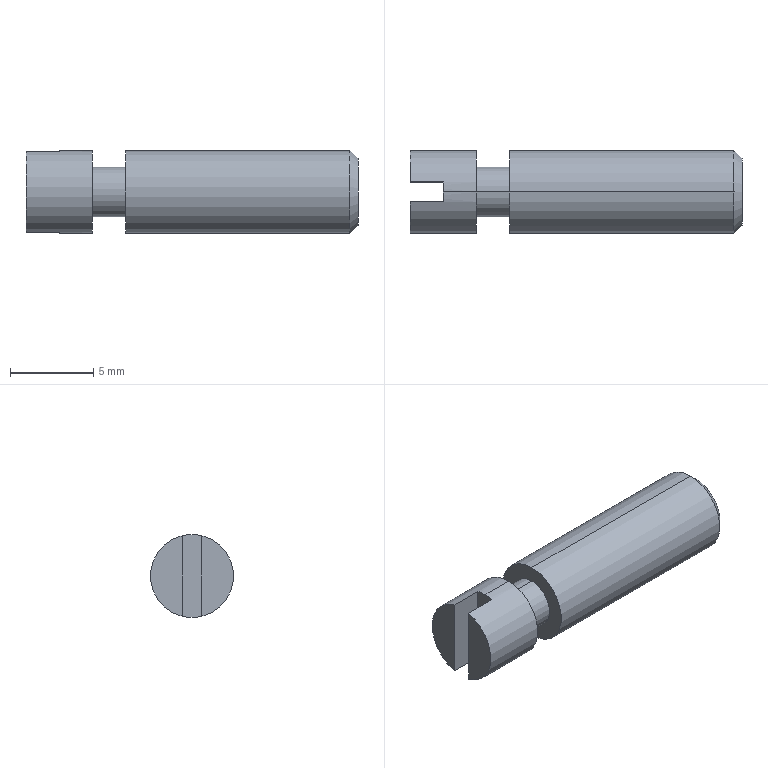Part | STEP file | QA-BSPO5_20b | 1 solid | 16 faces | box 20 x 5 x 5 mm | volume 353.917 mm3 | plane 8 | cylinder 6 | cone 2 | commonest cylinder face diameters 5 x4 3 x2
STEP:
#1=CARTESIAN_POINT('',(0.,0.,0.));
#2=DIRECTION('',(0.,0.,1.));
#3=DIRECTION('',(1.,0.,0.));
#4=AXIS2_PLACEMENT_3D('',#1,#2,#3);
#5=CARTESIAN_POINT('',(4.,0.,-2.5));
#6=VERTEX_POINT('',#5);
#7=CARTESIAN_POINT('',(4.,0.,2.5));
#8=VERTEX_POINT('',#7);
#9=CARTESIAN_POINT('',(4.,0.,0.));
#10=DIRECTION('',(1.,0.,0.));
#11=DIRECTION('',(0.,0.,-1.));
#12=AXIS2_PLACEMENT_3D('',#9,#10,#11);
#13=CIRCLE('',#12,2.5);
#14=CARTESIAN_POINT('',(20.,0.,0.));
#15=DIRECTION('',(-1.,0.,0.));
#16=DIRECTION('',(0.,0.,1.));
#17=AXIS2_PLACEMENT_3D('',#14,#15,#16);
#18=CYLINDRICAL_SURFACE('',#17,2.5);
#19=CARTESIAN_POINT('',(3.142,16.));
#20=DIRECTION('',(-1.,0.));
#21=VECTOR('',#20,1.);
#22=LINE('',#19,#21);
#23=(GEOMETRIC_REPRESENTATION_CONTEXT(2)PARAMETRIC_REPRESENTATION_CONTEXT()REPRESENTATION_CONTEXT('',''));
#24=DEFINITIONAL_REPRESENTATION('',(#22),#23);
#25=PCURVE('',#18,#24);
#26=CARTESIAN_POINT('',(4.,3.5,0.));
#27=DIRECTION('',(1.,0.,0.));
#28=DIRECTION('',(0.,0.,-1.));
#29=AXIS2_PLACEMENT_3D('',#26,#27,#28);
#30=PLANE('',#29);
#31=CARTESIAN_POINT('',(0.,-3.5));
#32=DIRECTION('',(1.,0.));
#33=AXIS2_PLACEMENT_2D('',#31,#32);
#34=CIRCLE('',#33,2.5);
#35=(GEOMETRIC_REPRESENTATION_CONTEXT(2)PARAMETRIC_REPRESENTATION_CONTEXT()REPRESENTATION_CONTEXT('',''));
#36=DEFINITIONAL_REPRESENTATION('',(#34),#35);
#37=PCURVE('',#30,#36);
#38=SURFACE_CURVE('',#13,(#25,#37),.PCURVE_S1.);
#39=EDGE_CURVE('',#6,#8,#38,.T.);
#40=ORIENTED_EDGE('',*,*,#39,.F.);
#41=CARTESIAN_POINT('',(2.,0.,-2.5));
#42=VERTEX_POINT('',#41);
#43=CARTESIAN_POINT('',(20.,0.,-2.5));
#44=DIRECTION('',(-1.,0.,0.));
#45=VECTOR('',#44,1.);
#46=LINE('',#43,#45);
#47=CARTESIAN_POINT('',(3.142,0.));
#48=DIRECTION('',(0.,1.));
#49=VECTOR('',#48,1.);
#50=LINE('',#47,#49);
#51=(GEOMETRIC_REPRESENTATION_CONTEXT(2)PARAMETRIC_REPRESENTATION_CONTEXT()REPRESENTATION_CONTEXT('',''));
#52=DEFINITIONAL_REPRESENTATION('',(#50),#51);
#53=PCURVE('',#18,#52);
#54=CARTESIAN_POINT('',(20.,0.,0.));
#55=DIRECTION('',(-1.,0.,0.));
#56=DIRECTION('',(0.,0.,1.));
#57=AXIS2_PLACEMENT_3D('',#54,#55,#56);
#58=CYLINDRICAL_SURFACE('',#57,2.5);
#59=CARTESIAN_POINT('',(3.142,0.));
#60=DIRECTION('',(0.,1.));
#61=VECTOR('',#60,1.);
#62=LINE('',#59,#61);
#63=(GEOMETRIC_REPRESENTATION_CONTEXT(2)PARAMETRIC_REPRESENTATION_CONTEXT()REPRESENTATION_CONTEXT('',''));
#64=DEFINITIONAL_REPRESENTATION('',(#62),#63);
#65=PCURVE('',#58,#64);
#66=SURFACE_CURVE('',#46,(#53,#65),.PCURVE_S1.);
#67=EDGE_CURVE('',#6,#42,#66,.T.);
#68=ORIENTED_EDGE('',*,*,#67,.T.);
#69=CARTESIAN_POINT('',(2.,0.6,-2.427));
#70=VERTEX_POINT('',#69);
#71=CARTESIAN_POINT('',(2.,0.,0.));
#72=DIRECTION('',(1.,0.,0.));
#73=DIRECTION('',(0.,0.,-1.));
#74=AXIS2_PLACEMENT_3D('',#71,#72,#73);
#75=CIRCLE('',#74,2.5);
#76=CARTESIAN_POINT('',(3.142,18.));
#77=DIRECTION('',(-1.,0.));
#78=VECTOR('',#77,1.);
#79=LINE('',#76,#78);
#80=(GEOMETRIC_REPRESENTATION_CONTEXT(2)PARAMETRIC_REPRESENTATION_CONTEXT()REPRESENTATION_CONTEXT('',''));
#81=DEFINITIONAL_REPRESENTATION('',(#79),#80);
#82=PCURVE('',#18,#81);
#83=CARTESIAN_POINT('',(2.,-0.6,-2.5));
#84=DIRECTION('',(1.,0.,0.));
#85=DIRECTION('',(0.,0.,-1.));
#86=AXIS2_PLACEMENT_3D('',#83,#84,#85);
#87=PLANE('',#86);
#88=CARTESIAN_POINT('',(-2.5,0.6));
#89=DIRECTION('',(1.,0.));
#90=AXIS2_PLACEMENT_2D('',#88,#89);
#91=CIRCLE('',#90,2.5);
#92=(GEOMETRIC_REPRESENTATION_CONTEXT(2)PARAMETRIC_REPRESENTATION_CONTEXT()REPRESENTATION_CONTEXT('',''));
#93=DEFINITIONAL_REPRESENTATION('',(#91),#92);
#94=PCURVE('',#87,#93);
#95=SURFACE_CURVE('',#75,(#82,#94),.PCURVE_S1.);
#96=EDGE_CURVE('',#42,#70,#95,.T.);
#97=ORIENTED_EDGE('',*,*,#96,.T.);
#98=CARTESIAN_POINT('',(0.,0.6,-2.427));
#99=VERTEX_POINT('',#98);
#100=CARTESIAN_POINT('',(20.,0.6,-2.427));
#101=DIRECTION('',(-1.,0.,0.));
#102=VECTOR('',#101,1.);
#103=LINE('',#100,#102);
#104=CARTESIAN_POINT('',(2.899,0.));
#105=DIRECTION('',(0.,1.));
#106=VECTOR('',#105,1.);
#107=LINE('',#104,#106);
#108=(GEOMETRIC_REPRESENTATION_CONTEXT(2)PARAMETRIC_REPRESENTATION_CONTEXT()REPRESENTATION_CONTEXT('',''));
#109=DEFINITIONAL_REPRESENTATION('',(#107),#108);
#110=PCURVE('',#18,#109);
#111=CARTESIAN_POINT('',(2.,0.6,-2.5));
#112=DIRECTION('',(0.,1.,0.));
#113=DIRECTION('',(0.,0.,1.));
#114=AXIS2_PLACEMENT_3D('',#111,#112,#113);
#115=PLANE('',#114);
#116=CARTESIAN_POINT('',(0.07307,18.));
#117=DIRECTION('',(0.,-1.));
#118=VECTOR('',#117,1.);
#119=LINE('',#116,#118);
#120=(GEOMETRIC_REPRESENTATION_CONTEXT(2)PARAMETRIC_REPRESENTATION_CONTEXT()REPRESENTATION_CONTEXT('',''));
#121=DEFINITIONAL_REPRESENTATION('',(#119),#120);
#122=PCURVE('',#115,#121);
#123=SURFACE_CURVE('',#103,(#110,#122),.PCURVE_S1.);
#124=EDGE_CURVE('',#70,#99,#123,.T.);
#125=ORIENTED_EDGE('',*,*,#124,.T.);
#126=CARTESIAN_POINT('',(0.,0.6,2.427));
#127=VERTEX_POINT('',#126);
#128=CARTESIAN_POINT('',(0.,0.,0.));
#129=DIRECTION('',(-1.,0.,0.));
#130=DIRECTION('',(0.,0.,1.));
#131=AXIS2_PLACEMENT_3D('',#128,#129,#130);
#132=CIRCLE('',#131,2.5);
#133=CARTESIAN_POINT('',(0.,20.));
#134=DIRECTION('',(1.,0.));
#135=VECTOR('',#134,1.);
#136=LINE('',#133,#135);
#137=(GEOMETRIC_REPRESENTATION_CONTEXT(2)PARAMETRIC_REPRESENTATION_CONTEXT()REPRESENTATION_CONTEXT('',''));
#138=DEFINITIONAL_REPRESENTATION('',(#136),#137);
#139=PCURVE('',#18,#138);
#140=CARTESIAN_POINT('',(0.,0.,0.));
#141=DIRECTION('',(1.,0.,0.));
#142=DIRECTION('',(0.,0.,-1.));
#143=AXIS2_PLACEMENT_3D('',#140,#141,#142);
#144=PLANE('',#143);
#145=CARTESIAN_POINT('',(-2.5,0.));
#146=CARTESIAN_POINT('',(-2.5,4.33));
#147=CARTESIAN_POINT('',(1.25,2.165));
#148=CARTESIAN_POINT('',(5.,0.));
#149=CARTESIAN_POINT('',(1.25,-2.165));
#150=CARTESIAN_POINT('',(-2.5,-4.33));
#151=CARTESIAN_POINT('',(-2.5,0.));
#152=(BOUNDED_CURVE()B_SPLINE_CURVE(2,(#145,#146,#147,#148,#149,#150,#151),.UNSPECIFIED.,.T.,.F.)B_SPLINE_CURVE_WITH_KNOTS((1,2,2,2,2,1),(-2.094,0.,2.094,4.189,6.283,8.378),.UNSPECIFIED.)CURVE()GEOMETRIC_REPRESENTATION_ITEM()RATIONAL_B_SPLINE_CURVE((1.,0.5,1.,0.5,1.,0.5,1.))REPRESENTATION_ITEM(''));
#153=(GEOMETRIC_REPRESENTATION_CONTEXT(2)PARAMETRIC_REPRESENTATION_CONTEXT()REPRESENTATION_CONTEXT('',''));
#154=DEFINITIONAL_REPRESENTATION('',(#152),#153);
#155=PCURVE('',#144,#154);
#156=SURFACE_CURVE('',#132,(#139,#155),.PCURVE_S1.);
#157=EDGE_CURVE('',#127,#99,#156,.T.);
#158=ORIENTED_EDGE('',*,*,#157,.F.);
#159=CARTESIAN_POINT('',(2.,0.6,2.427));
#160=VERTEX_POINT('',#159);
#161=CARTESIAN_POINT('',(20.,0.6,2.427));
#162=DIRECTION('',(1.,0.,0.));
#163=VECTOR('',#162,1.);
#164=LINE('',#161,#163);
#165=CARTESIAN_POINT('',(0.2424,0.));
#166=DIRECTION('',(0.,-1.));
#167=VECTOR('',#166,1.);
#168=LINE('',#165,#167);
#169=(GEOMETRIC_REPRESENTATION_CONTEXT(2)PARAMETRIC_REPRESENTATION_CONTEXT()REPRESENTATION_CONTEXT('',''));
#170=DEFINITIONAL_REPRESENTATION('',(#168),#169);
#171=PCURVE('',#18,#170);
#172=CARTESIAN_POINT('',(4.927,18.));
#173=DIRECTION('',(0.,1.));
#174=VECTOR('',#173,1.);
#175=LINE('',#172,#174);
#176=(GEOMETRIC_REPRESENTATION_CONTEXT(2)PARAMETRIC_REPRESENTATION_CONTEXT()REPRESENTATION_CONTEXT('',''));
#177=DEFINITIONAL_REPRESENTATION('',(#175),#176);
#178=PCURVE('',#115,#177);
#179=SURFACE_CURVE('',#164,(#171,#178),.PCURVE_S1.);
#180=EDGE_CURVE('',#127,#160,#179,.T.);
#181=ORIENTED_EDGE('',*,*,#180,.T.);
#182=CARTESIAN_POINT('',(2.,0.,2.5));
#183=VERTEX_POINT('',#182);
#184=CARTESIAN_POINT('',(2.,0.,0.));
#185=DIRECTION('',(1.,0.,0.));
#186=DIRECTION('',(0.,0.,-1.));
#187=AXIS2_PLACEMENT_3D('',#184,#185,#186);
#188=CIRCLE('',#187,2.5);
#189=CARTESIAN_POINT('',(3.142,18.));
#190=DIRECTION('',(-1.,0.));
#191=VECTOR('',#190,1.);
#192=LINE('',#189,#191);
#193=(GEOMETRIC_REPRESENTATION_CONTEXT(2)PARAMETRIC_REPRESENTATION_CONTEXT()REPRESENTATION_CONTEXT('',''));
#194=DEFINITIONAL_REPRESENTATION('',(#192),#193);
#195=PCURVE('',#18,#194);
#196=CARTESIAN_POINT('',(-2.5,0.6));
#197=DIRECTION('',(1.,0.));
#198=AXIS2_PLACEMENT_2D('',#196,#197);
#199=CIRCLE('',#198,2.5);
#200=(GEOMETRIC_REPRESENTATION_CONTEXT(2)PARAMETRIC_REPRESENTATION_CONTEXT()REPRESENTATION_CONTEXT('',''));
#201=DEFINITIONAL_REPRESENTATION('',(#199),#200);
#202=PCURVE('',#87,#201);
#203=SURFACE_CURVE('',#188,(#195,#202),.PCURVE_S1.);
#204=EDGE_CURVE('',#160,#183,#203,.T.);
#205=ORIENTED_EDGE('',*,*,#204,.T.);
#206=CARTESIAN_POINT('',(20.,0.,2.5));
#207=DIRECTION('',(-1.,0.,0.));
#208=VECTOR('',#207,1.);
#209=LINE('',#206,#208);
#210=CARTESIAN_POINT('',(0.,0.));
#211=DIRECTION('',(0.,1.));
#212=VECTOR('',#211,1.);
#213=LINE('',#210,#212);
#214=(GEOMETRIC_REPRESENTATION_CONTEXT(2)PARAMETRIC_REPRESENTATION_CONTEXT()REPRESENTATION_CONTEXT('',''));
#215=DEFINITIONAL_REPRESENTATION('',(#213),#214);
#216=PCURVE('',#18,#215);
#217=CARTESIAN_POINT('',(6.283,0.));
#218=DIRECTION('',(0.,1.));
#219=VECTOR('',#218,1.);
#220=LINE('',#217,#219);
#221=(GEOMETRIC_REPRESENTATION_CONTEXT(2)PARAMETRIC_REPRESENTATION_CONTEXT()REPRESENTATION_CONTEXT('',''));
#222=DEFINITIONAL_REPRESENTATION('',(#220),#221);
#223=PCURVE('',#58,#222);
#224=SURFACE_CURVE('',#209,(#216,#223),.PCURVE_S1.);
#225=EDGE_CURVE('',#8,#183,#224,.T.);
#226=ORIENTED_EDGE('',*,*,#225,.F.);
#227=EDGE_LOOP('',(#40,#68,#97,#125,#158,#181,#205,#226));
#228=FACE_BOUND('',#227,.T.);
#229=ADVANCED_FACE('',(#228),#18,.T.);
#230=CARTESIAN_POINT('',(6.,0.,1.5));
#231=VERTEX_POINT('',#230);
#232=CARTESIAN_POINT('',(6.,0.,-1.5));
#233=VERTEX_POINT('',#232);
#234=CARTESIAN_POINT('',(6.,0.,0.));
#235=DIRECTION('',(-1.,0.,0.));
#236=DIRECTION('',(0.,0.,1.));
#237=AXIS2_PLACEMENT_3D('',#234,#235,#236);
#238=CIRCLE('',#237,1.5);
#239=CARTESIAN_POINT('',(5.,0.,0.));
#240=DIRECTION('',(-1.,0.,0.));
#241=DIRECTION('',(0.,0.,1.));
#242=AXIS2_PLACEMENT_3D('',#239,#240,#241);
#243=CYLINDRICAL_SURFACE('',#242,1.5);
#244=CARTESIAN_POINT('',(0.,-1.));
#245=DIRECTION('',(1.,0.));
#246=VECTOR('',#245,1.);
#247=LINE('',#244,#246);
#248=(GEOMETRIC_REPRESENTATION_CONTEXT(2)PARAMETRIC_REPRESENTATION_CONTEXT()REPRESENTATION_CONTEXT('',''));
#249=DEFINITIONAL_REPRESENTATION('',(#247),#248);
#250=PCURVE('',#243,#249);
#251=CARTESIAN_POINT('',(6.,1.5,0.));
#252=DIRECTION('',(-1.,0.,0.));
#253=DIRECTION('',(0.,0.,1.));
#254=AXIS2_PLACEMENT_3D('',#251,#252,#253);
#255=PLANE('',#254);
#256=CARTESIAN_POINT('',(0.,-1.5));
#257=DIRECTION('',(1.,0.));
#258=AXIS2_PLACEMENT_2D('',#256,#257);
#259=CIRCLE('',#258,1.5);
#260=(GEOMETRIC_REPRESENTATION_CONTEXT(2)PARAMETRIC_REPRESENTATION_CONTEXT()REPRESENTATION_CONTEXT('',''));
#261=DEFINITIONAL_REPRESENTATION('',(#259),#260);
#262=PCURVE('',#255,#261);
#263=SURFACE_CURVE('',#238,(#250,#262),.PCURVE_S1.);
#264=EDGE_CURVE('',#231,#233,#263,.T.);
#265=ORIENTED_EDGE('',*,*,#264,.T.);
#266=CARTESIAN_POINT('',(4.,0.,-1.5));
#267=VERTEX_POINT('',#266);
#268=CARTESIAN_POINT('',(5.,0.,-1.5));
#269=DIRECTION('',(-1.,0.,0.));
#270=VECTOR('',#269,1.);
#271=LINE('',#268,#270);
#272=CARTESIAN_POINT('',(3.142,0.));
#273=DIRECTION('',(0.,1.));
#274=VECTOR('',#273,1.);
#275=LINE('',#272,#274);
#276=(GEOMETRIC_REPRESENTATION_CONTEXT(2)PARAMETRIC_REPRESENTATION_CONTEXT()REPRESENTATION_CONTEXT('',''));
#277=DEFINITIONAL_REPRESENTATION('',(#275),#276);
#278=PCURVE('',#243,#277);
#279=CARTESIAN_POINT('',(5.,0.,0.));
#280=DIRECTION('',(-1.,0.,0.));
#281=DIRECTION('',(0.,0.,1.));
#282=AXIS2_PLACEMENT_3D('',#279,#280,#281);
#283=CYLINDRICAL_SURFACE('',#282,1.5);
#284=CARTESIAN_POINT('',(3.142,0.));
#285=DIRECTION('',(0.,1.));
#286=VECTOR('',#285,1.);
#287=LINE('',#284,#286);
#288=(GEOMETRIC_REPRESENTATION_CONTEXT(2)PARAMETRIC_REPRESENTATION_CONTEXT()REPRESENTATION_CONTEXT('',''));
#289=DEFINITIONAL_REPRESENTATION('',(#287),#288);
#290=PCURVE('',#283,#289);
#291=SURFACE_CURVE('',#271,(#278,#290),.PCURVE_S1.);
#292=EDGE_CURVE('',#233,#267,#291,.T.);
#293=ORIENTED_EDGE('',*,*,#292,.T.);
#294=CARTESIAN_POINT('',(4.,0.,1.5));
#295=VERTEX_POINT('',#294);
#296=CARTESIAN_POINT('',(4.,0.,0.));
#297=DIRECTION('',(-1.,0.,0.));
#298=DIRECTION('',(0.,0.,1.));
#299=AXIS2_PLACEMENT_3D('',#296,#297,#298);
#300=CIRCLE('',#299,1.5);
#301=CARTESIAN_POINT('',(0.,1.));
#302=DIRECTION('',(1.,0.));
#303=VECTOR('',#302,1.);
#304=LINE('',#301,#303);
#305=(GEOMETRIC_REPRESENTATION_CONTEXT(2)PARAMETRIC_REPRESENTATION_CONTEXT()REPRESENTATION_CONTEXT('',''));
#306=DEFINITIONAL_REPRESENTATION('',(#304),#305);
#307=PCURVE('',#243,#306);
#308=CARTESIAN_POINT('',(-1.5,-3.5));
#309=CARTESIAN_POINT('',(-1.5,-0.9019));
#310=CARTESIAN_POINT('',(0.75,-2.201));
#311=CARTESIAN_POINT('',(3.,-3.5));
#312=CARTESIAN_POINT('',(0.75,-4.799));
#313=CARTESIAN_POINT('',(-1.5,-6.098));
#314=CARTESIAN_POINT('',(-1.5,-3.5));
#315=(BOUNDED_CURVE()B_SPLINE_CURVE(2,(#308,#309,#310,#311,#312,#313,#314),.UNSPECIFIED.,.T.,.F.)B_SPLINE_CURVE_WITH_KNOTS((1,2,2,2,2,1),(-2.094,0.,2.094,4.189,6.283,8.378),.UNSPECIFIED.)CURVE()GEOMETRIC_REPRESENTATION_ITEM()RATIONAL_B_SPLINE_CURVE((1.,0.5,1.,0.5,1.,0.5,1.))REPRESENTATION_ITEM(''));
#316=(GEOMETRIC_REPRESENTATION_CONTEXT(2)PARAMETRIC_REPRESENTATION_CONTEXT()REPRESENTATION_CONTEXT('',''));
#317=DEFINITIONAL_REPRESENTATION('',(#315),#316);
#318=PCURVE('',#30,#317);
#319=SURFACE_CURVE('',#300,(#307,#318),.PCURVE_S1.);
#320=EDGE_CURVE('',#295,#267,#319,.T.);
#321=ORIENTED_EDGE('',*,*,#320,.F.);
#322=CARTESIAN_POINT('',(5.,0.,1.5));
#323=DIRECTION('',(-1.,0.,0.));
#324=VECTOR('',#323,1.);
#325=LINE('',#322,#324);
#326=CARTESIAN_POINT('',(0.,0.));
#327=DIRECTION('',(0.,1.));
#328=VECTOR('',#327,1.);
#329=LINE('',#326,#328);
#330=(GEOMETRIC_REPRESENTATION_CONTEXT(2)PARAMETRIC_REPRESENTATION_CONTEXT()REPRESENTATION_CONTEXT('',''));
#331=DEFINITIONAL_REPRESENTATION('',(#329),#330);
#332=PCURVE('',#243,#331);
#333=CARTESIAN_POINT('',(6.283,0.));
#334=DIRECTION('',(0.,1.));
#335=VECTOR('',#334,1.);
#336=LINE('',#333,#335);
#337=(GEOMETRIC_REPRESENTATION_CONTEXT(2)PARAMETRIC_REPRESENTATION_CONTEXT()REPRESENTATION_CONTEXT('',''));
#338=DEFINITIONAL_REPRESENTATION('',(#336),#337);
#339=PCURVE('',#283,#338);
#340=SURFACE_CURVE('',#325,(#332,#339),.PCURVE_S1.);
#341=EDGE_CURVE('',#231,#295,#340,.T.);
#342=ORIENTED_EDGE('',*,*,#341,.F.);
#343=EDGE_LOOP('',(#265,#293,#321,#342));
#344=FACE_BOUND('',#343,.T.);
#345=ADVANCED_FACE('',(#344),#243,.T.);
#346=CARTESIAN_POINT('',(20.,0.,2.01));
#347=VERTEX_POINT('',#346);
#348=CARTESIAN_POINT('',(20.,0.,-2.01));
#349=VERTEX_POINT('',#348);
#350=CARTESIAN_POINT('',(20.,0.,0.));
#351=DIRECTION('',(-1.,0.,0.));
#352=DIRECTION('',(0.,0.,1.));
#353=AXIS2_PLACEMENT_3D('',#350,#351,#352);
#354=CIRCLE('',#353,2.01);
#355=CARTESIAN_POINT('',(20.,0.,0.));
#356=DIRECTION('',(-1.,0.,0.));
#357=DIRECTION('',(0.,0.,1.));
#358=AXIS2_PLACEMENT_3D('',#355,#356,#357);
#359=CONICAL_SURFACE('',#358,2.01,0.7854);
#360=CARTESIAN_POINT('',(0.,0.));
#361=DIRECTION('',(1.,0.));
#362=VECTOR('',#361,1.);
#363=LINE('',#360,#362);
#364=(GEOMETRIC_REPRESENTATION_CONTEXT(2)PARAMETRIC_REPRESENTATION_CONTEXT()REPRESENTATION_CONTEXT('',''));
#365=DEFINITIONAL_REPRESENTATION('',(#363),#364);
#366=PCURVE('',#359,#365);
#367=CARTESIAN_POINT('',(20.,2.01,0.));
#368=DIRECTION('',(-1.,0.,0.));
#369=DIRECTION('',(0.,0.,1.));
#370=AXIS2_PLACEMENT_3D('',#367,#368,#369);
#371=PLANE('',#370);
#372=CARTESIAN_POINT('',(0.,-2.01));
#373=DIRECTION('',(1.,0.));
#374=AXIS2_PLACEMENT_2D('',#372,#373);
#375=CIRCLE('',#374,2.01);
#376=(GEOMETRIC_REPRESENTATION_CONTEXT(2)PARAMETRIC_REPRESENTATION_CONTEXT()REPRESENTATION_CONTEXT('',''));
#377=DEFINITIONAL_REPRESENTATION('',(#375),#376);
#378=PCURVE('',#371,#377);
#379=SURFACE_CURVE('',#354,(#366,#378),.PCURVE_S1.);
#380=EDGE_CURVE('',#347,#349,#379,.T.);
#381=ORIENTED_EDGE('',*,*,#380,.T.);
#382=CARTESIAN_POINT('',(19.509,0.,-2.5));
#383=VERTEX_POINT('',#382);
#384=CARTESIAN_POINT('',(20.,0.,-2.01));
#385=DIRECTION('',(-0.7071,0.,-0.7071));
#386=VECTOR('',#385,1.);
#387=LINE('',#384,#386);
#388=CARTESIAN_POINT('',(3.142,0.));
#389=DIRECTION('',(0.,1.));
#390=VECTOR('',#389,1.);
#391=LINE('',#388,#390);
#392=(GEOMETRIC_REPRESENTATION_CONTEXT(2)PARAMETRIC_REPRESENTATION_CONTEXT()REPRESENTATION_CONTEXT('',''));
#393=DEFINITIONAL_REPRESENTATION('',(#391),#392);
#394=PCURVE('',#359,#393);
#395=CARTESIAN_POINT('',(20.,0.,0.));
#396=DIRECTION('',(-1.,0.,0.));
#397=DIRECTION('',(0.,0.,1.));
#398=AXIS2_PLACEMENT_3D('',#395,#396,#397);
#399=CONICAL_SURFACE('',#398,2.01,0.7854);
#400=CARTESIAN_POINT('',(3.142,0.));
#401=DIRECTION('',(0.,1.));
#402=VECTOR('',#401,1.);
#403=LINE('',#400,#402);
#404=(GEOMETRIC_REPRESENTATION_CONTEXT(2)PARAMETRIC_REPRESENTATION_CONTEXT()REPRESENTATION_CONTEXT('',''));
#405=DEFINITIONAL_REPRESENTATION('',(#403),#404);
#406=PCURVE('',#399,#405);
#407=SURFACE_CURVE('',#387,(#394,#406),.PCURVE_S1.);
#408=EDGE_CURVE('',#349,#383,#407,.T.);
#409=ORIENTED_EDGE('',*,*,#408,.T.);
#410=CARTESIAN_POINT('',(19.509,0.,2.5));
#411=VERTEX_POINT('',#410);
#412=CARTESIAN_POINT('',(19.509,0.,0.));
#413=DIRECTION('',(-1.,0.,0.));
#414=DIRECTION('',(0.,0.,1.));
#415=AXIS2_PLACEMENT_3D('',#412,#413,#414);
#416=CIRCLE('',#415,2.5);
#417=CARTESIAN_POINT('',(0.,0.4905));
#418=DIRECTION('',(1.,0.));
#419=VECTOR('',#418,1.);
#420=LINE('',#417,#419);
#421=(GEOMETRIC_REPRESENTATION_CONTEXT(2)PARAMETRIC_REPRESENTATION_CONTEXT()REPRESENTATION_CONTEXT('',''));
#422=DEFINITIONAL_REPRESENTATION('',(#420),#421);
#423=PCURVE('',#359,#422);
#424=CARTESIAN_POINT('',(20.,0.,0.));
#425=DIRECTION('',(-1.,0.,0.));
#426=DIRECTION('',(0.,0.,1.));
#427=AXIS2_PLACEMENT_3D('',#424,#425,#426);
#428=CYLINDRICAL_SURFACE('',#427,2.5);
#429=CARTESIAN_POINT('',(0.,0.4905));
#430=DIRECTION('',(1.,0.));
#431=VECTOR('',#430,1.);
#432=LINE('',#429,#431);
#433=(GEOMETRIC_REPRESENTATION_CONTEXT(2)PARAMETRIC_REPRESENTATION_CONTEXT()REPRESENTATION_CONTEXT('',''));
#434=DEFINITIONAL_REPRESENTATION('',(#432),#433);
#435=PCURVE('',#428,#434);
#436=SURFACE_CURVE('',#416,(#423,#435),.PCURVE_S1.);
#437=EDGE_CURVE('',#411,#383,#436,.T.);
#438=ORIENTED_EDGE('',*,*,#437,.F.);
#439=CARTESIAN_POINT('',(20.,0.,2.01));
#440=DIRECTION('',(-0.7071,0.,0.7071));
#441=VECTOR('',#440,1.);
#442=LINE('',#439,#441);
#443=CARTESIAN_POINT('',(0.,0.));
#444=DIRECTION('',(0.,1.));
#445=VECTOR('',#444,1.);
#446=LINE('',#443,#445);
#447=(GEOMETRIC_REPRESENTATION_CONTEXT(2)PARAMETRIC_REPRESENTATION_CONTEXT()REPRESENTATION_CONTEXT('',''));
#448=DEFINITIONAL_REPRESENTATION('',(#446),#447);
#449=PCURVE('',#359,#448);
#450=CARTESIAN_POINT('',(6.283,0.));
#451=DIRECTION('',(0.,1.));
#452=VECTOR('',#451,1.);
#453=LINE('',#450,#452);
#454=(GEOMETRIC_REPRESENTATION_CONTEXT(2)PARAMETRIC_REPRESENTATION_CONTEXT()REPRESENTATION_CONTEXT('',''));
#455=DEFINITIONAL_REPRESENTATION('',(#453),#454);
#456=PCURVE('',#399,#455);
#457=SURFACE_CURVE('',#442,(#449,#456),.PCURVE_S1.);
#458=EDGE_CURVE('',#347,#411,#457,.T.);
#459=ORIENTED_EDGE('',*,*,#458,.F.);
#460=EDGE_LOOP('',(#381,#409,#438,#459));
#461=FACE_BOUND('',#460,.T.);
#462=ADVANCED_FACE('',(#461),#359,.T.);
#463=ORIENTED_EDGE('',*,*,#437,.T.);
#464=CARTESIAN_POINT('',(6.,0.,-2.5));
#465=VERTEX_POINT('',#464);
#466=CARTESIAN_POINT('',(20.,0.,-2.5));
#467=DIRECTION('',(-1.,0.,0.));
#468=VECTOR('',#467,1.);
#469=LINE('',#466,#468);
#470=CARTESIAN_POINT('',(3.142,0.));
#471=DIRECTION('',(0.,1.));
#472=VECTOR('',#471,1.);
#473=LINE('',#470,#472);
#474=(GEOMETRIC_REPRESENTATION_CONTEXT(2)PARAMETRIC_REPRESENTATION_CONTEXT()REPRESENTATION_CONTEXT('',''));
#475=DEFINITIONAL_REPRESENTATION('',(#473),#474);
#476=PCURVE('',#428,#475);
#477=CARTESIAN_POINT('',(20.,0.,0.));
#478=DIRECTION('',(-1.,0.,0.));
#479=DIRECTION('',(0.,0.,1.));
#480=AXIS2_PLACEMENT_3D('',#477,#478,#479);
#481=CYLINDRICAL_SURFACE('',#480,2.5);
#482=CARTESIAN_POINT('',(3.142,0.));
#483=DIRECTION('',(0.,1.));
#484=VECTOR('',#483,1.);
#485=LINE('',#482,#484);
#486=(GEOMETRIC_REPRESENTATION_CONTEXT(2)PARAMETRIC_REPRESENTATION_CONTEXT()REPRESENTATION_CONTEXT('',''));
#487=DEFINITIONAL_REPRESENTATION('',(#485),#486);
#488=PCURVE('',#481,#487);
#489=SURFACE_CURVE('',#469,(#476,#488),.PCURVE_S1.);
#490=EDGE_CURVE('',#383,#465,#489,.T.);
#491=ORIENTED_EDGE('',*,*,#490,.T.);
#492=CARTESIAN_POINT('',(6.,0.,2.5));
#493=VERTEX_POINT('',#492);
#494=CARTESIAN_POINT('',(6.,0.,0.));
#495=DIRECTION('',(-1.,0.,0.));
#496=DIRECTION('',(0.,0.,1.));
#497=AXIS2_PLACEMENT_3D('',#494,#495,#496);
#498=CIRCLE('',#497,2.5);
#499=CARTESIAN_POINT('',(0.,14.));
#500=DIRECTION('',(1.,0.));
#501=VECTOR('',#500,1.);
#502=LINE('',#499,#501);
#503=(GEOMETRIC_REPRESENTATION_CONTEXT(2)PARAMETRIC_REPRESENTATION_CONTEXT()REPRESENTATION_CONTEXT('',''));
#504=DEFINITIONAL_REPRESENTATION('',(#502),#503);
#505=PCURVE('',#428,#504);
#506=CARTESIAN_POINT('',(0.,-1.5));
#507=DIRECTION('',(1.,0.));
#508=AXIS2_PLACEMENT_2D('',#506,#507);
#509=CIRCLE('',#508,2.5);
#510=(GEOMETRIC_REPRESENTATION_CONTEXT(2)PARAMETRIC_REPRESENTATION_CONTEXT()REPRESENTATION_CONTEXT('',''));
#511=DEFINITIONAL_REPRESENTATION('',(#509),#510);
#512=PCURVE('',#255,#511);
#513=SURFACE_CURVE('',#498,(#505,#512),.PCURVE_S1.);
#514=EDGE_CURVE('',#493,#465,#513,.T.);
#515=ORIENTED_EDGE('',*,*,#514,.F.);
#516=CARTESIAN_POINT('',(20.,0.,2.5));
#517=DIRECTION('',(-1.,0.,0.));
#518=VECTOR('',#517,1.);
#519=LINE('',#516,#518);
#520=CARTESIAN_POINT('',(0.,0.));
#521=DIRECTION('',(0.,1.));
#522=VECTOR('',#521,1.);
#523=LINE('',#520,#522);
#524=(GEOMETRIC_REPRESENTATION_CONTEXT(2)PARAMETRIC_REPRESENTATION_CONTEXT()REPRESENTATION_CONTEXT('',''));
#525=DEFINITIONAL_REPRESENTATION('',(#523),#524);
#526=PCURVE('',#428,#525);
#527=CARTESIAN_POINT('',(6.283,0.));
#528=DIRECTION('',(0.,1.));
#529=VECTOR('',#528,1.);
#530=LINE('',#527,#529);
#531=(GEOMETRIC_REPRESENTATION_CONTEXT(2)PARAMETRIC_REPRESENTATION_CONTEXT()REPRESENTATION_CONTEXT('',''));
#532=DEFINITIONAL_REPRESENTATION('',(#530),#531);
#533=PCURVE('',#481,#532);
#534=SURFACE_CURVE('',#519,(#526,#533),.PCURVE_S1.);
#535=EDGE_CURVE('',#411,#493,#534,.T.);
#536=ORIENTED_EDGE('',*,*,#535,.F.);
#537=EDGE_LOOP('',(#463,#491,#515,#536));
#538=FACE_BOUND('',#537,.T.);
#539=ADVANCED_FACE('',(#538),#428,.T.);
#540=ORIENTED_EDGE('',*,*,#490,.F.);
#541=CARTESIAN_POINT('',(19.509,0.,0.));
#542=DIRECTION('',(-1.,0.,0.));
#543=DIRECTION('',(0.,0.,1.));
#544=AXIS2_PLACEMENT_3D('',#541,#542,#543);
#545=CIRCLE('',#544,2.5);
#546=CARTESIAN_POINT('',(0.,0.4905));
#547=DIRECTION('',(1.,0.));
#548=VECTOR('',#547,1.);
#549=LINE('',#546,#548);
#550=(GEOMETRIC_REPRESENTATION_CONTEXT(2)PARAMETRIC_REPRESENTATION_CONTEXT()REPRESENTATION_CONTEXT('',''));
#551=DEFINITIONAL_REPRESENTATION('',(#549),#550);
#552=PCURVE('',#481,#551);
#553=CARTESIAN_POINT('',(0.,0.4905));
#554=DIRECTION('',(1.,0.));
#555=VECTOR('',#554,1.);
#556=LINE('',#553,#555);
#557=(GEOMETRIC_REPRESENTATION_CONTEXT(2)PARAMETRIC_REPRESENTATION_CONTEXT()REPRESENTATION_CONTEXT('',''));
#558=DEFINITIONAL_REPRESENTATION('',(#556),#557);
#559=PCURVE('',#399,#558);
#560=SURFACE_CURVE('',#545,(#552,#559),.PCURVE_S1.);
#561=EDGE_CURVE('',#383,#411,#560,.T.);
#562=ORIENTED_EDGE('',*,*,#561,.T.);
#563=ORIENTED_EDGE('',*,*,#535,.T.);
#564=CARTESIAN_POINT('',(6.,0.,0.));
#565=DIRECTION('',(-1.,0.,0.));
#566=DIRECTION('',(0.,0.,1.));
#567=AXIS2_PLACEMENT_3D('',#564,#565,#566);
#568=CIRCLE('',#567,2.5);
#569=CARTESIAN_POINT('',(0.,14.));
#570=DIRECTION('',(1.,0.));
#571=VECTOR('',#570,1.);
#572=LINE('',#569,#571);
#573=(GEOMETRIC_REPRESENTATION_CONTEXT(2)PARAMETRIC_REPRESENTATION_CONTEXT()REPRESENTATION_CONTEXT('',''));
#574=DEFINITIONAL_REPRESENTATION('',(#572),#573);
#575=PCURVE('',#481,#574);
#576=CARTESIAN_POINT('',(0.,-1.5));
#577=DIRECTION('',(1.,0.));
#578=AXIS2_PLACEMENT_2D('',#576,#577);
#579=CIRCLE('',#578,2.5);
#580=(GEOMETRIC_REPRESENTATION_CONTEXT(2)PARAMETRIC_REPRESENTATION_CONTEXT()REPRESENTATION_CONTEXT('',''));
#581=DEFINITIONAL_REPRESENTATION('',(#579),#580);
#582=PCURVE('',#255,#581);
#583=SURFACE_CURVE('',#568,(#575,#582),.PCURVE_S1.);
#584=EDGE_CURVE('',#465,#493,#583,.T.);
#585=ORIENTED_EDGE('',*,*,#584,.F.);
#586=EDGE_LOOP('',(#540,#562,#563,#585));
#587=FACE_BOUND('',#586,.T.);
#588=ADVANCED_FACE('',(#587),#481,.T.);
#589=ORIENTED_EDGE('',*,*,#408,.F.);
#590=CARTESIAN_POINT('',(20.,0.,0.));
#591=DIRECTION('',(-1.,0.,0.));
#592=DIRECTION('',(0.,0.,1.));
#593=AXIS2_PLACEMENT_3D('',#590,#591,#592);
#594=CIRCLE('',#593,2.01);
#595=CARTESIAN_POINT('',(0.,0.));
#596=DIRECTION('',(1.,0.));
#597=VECTOR('',#596,1.);
#598=LINE('',#595,#597);
#599=(GEOMETRIC_REPRESENTATION_CONTEXT(2)PARAMETRIC_REPRESENTATION_CONTEXT()REPRESENTATION_CONTEXT('',''));
#600=DEFINITIONAL_REPRESENTATION('',(#598),#599);
#601=PCURVE('',#399,#600);
#602=CARTESIAN_POINT('',(0.,-2.01));
#603=DIRECTION('',(1.,0.));
#604=AXIS2_PLACEMENT_2D('',#602,#603);
#605=CIRCLE('',#604,2.01);
#606=(GEOMETRIC_REPRESENTATION_CONTEXT(2)PARAMETRIC_REPRESENTATION_CONTEXT()REPRESENTATION_CONTEXT('',''));
#607=DEFINITIONAL_REPRESENTATION('',(#605),#606);
#608=PCURVE('',#371,#607);
#609=SURFACE_CURVE('',#594,(#601,#608),.PCURVE_S1.);
#610=EDGE_CURVE('',#349,#347,#609,.T.);
#611=ORIENTED_EDGE('',*,*,#610,.T.);
#612=ORIENTED_EDGE('',*,*,#458,.T.);
#613=ORIENTED_EDGE('',*,*,#561,.F.);
#614=EDGE_LOOP('',(#589,#611,#612,#613));
#615=FACE_BOUND('',#614,.T.);
#616=ADVANCED_FACE('',(#615),#399,.T.);
#617=ORIENTED_EDGE('',*,*,#380,.F.);
#618=ORIENTED_EDGE('',*,*,#610,.F.);
#619=EDGE_LOOP('',(#617,#618));
#620=FACE_BOUND('',#619,.T.);
#621=ADVANCED_FACE('',(#620),#371,.F.);
#622=ORIENTED_EDGE('',*,*,#320,.T.);
#623=CARTESIAN_POINT('',(4.,0.,0.));
#624=DIRECTION('',(-1.,0.,0.));
#625=DIRECTION('',(0.,0.,1.));
#626=AXIS2_PLACEMENT_3D('',#623,#624,#625);
#627=CIRCLE('',#626,1.5);
#628=CARTESIAN_POINT('',(-1.5,-3.5));
#629=CARTESIAN_POINT('',(-1.5,-0.9019));
#630=CARTESIAN_POINT('',(0.75,-2.201));
#631=CARTESIAN_POINT('',(3.,-3.5));
#632=CARTESIAN_POINT('',(0.75,-4.799));
#633=CARTESIAN_POINT('',(-1.5,-6.098));
#634=CARTESIAN_POINT('',(-1.5,-3.5));
#635=(BOUNDED_CURVE()B_SPLINE_CURVE(2,(#628,#629,#630,#631,#632,#633,#634),.UNSPECIFIED.,.T.,.F.)B_SPLINE_CURVE_WITH_KNOTS((1,2,2,2,2,1),(-2.094,0.,2.094,4.189,6.283,8.378),.UNSPECIFIED.)CURVE()GEOMETRIC_REPRESENTATION_ITEM()RATIONAL_B_SPLINE_CURVE((1.,0.5,1.,0.5,1.,0.5,1.))REPRESENTATION_ITEM(''));
#636=(GEOMETRIC_REPRESENTATION_CONTEXT(2)PARAMETRIC_REPRESENTATION_CONTEXT()REPRESENTATION_CONTEXT('',''));
#637=DEFINITIONAL_REPRESENTATION('',(#635),#636);
#638=PCURVE('',#30,#637);
#639=CARTESIAN_POINT('',(0.,1.));
#640=DIRECTION('',(1.,0.));
#641=VECTOR('',#640,1.);
#642=LINE('',#639,#641);
#643=(GEOMETRIC_REPRESENTATION_CONTEXT(2)PARAMETRIC_REPRESENTATION_CONTEXT()REPRESENTATION_CONTEXT('',''));
#644=DEFINITIONAL_REPRESENTATION('',(#642),#643);
#645=PCURVE('',#283,#644);
#646=SURFACE_CURVE('',#627,(#638,#645),.PCURVE_S1.);
#647=EDGE_CURVE('',#267,#295,#646,.T.);
#648=ORIENTED_EDGE('',*,*,#647,.T.);
#649=EDGE_LOOP('',(#622,#648));
#650=FACE_BOUND('',#649,.T.);
#651=CARTESIAN_POINT('',(4.,0.,0.));
#652=DIRECTION('',(1.,0.,0.));
#653=DIRECTION('',(0.,0.,-1.));
#654=AXIS2_PLACEMENT_3D('',#651,#652,#653);
#655=CIRCLE('',#654,2.5);
#656=CARTESIAN_POINT('',(0.,-3.5));
#657=DIRECTION('',(1.,0.));
#658=AXIS2_PLACEMENT_2D('',#656,#657);
#659=CIRCLE('',#658,2.5);
#660=(GEOMETRIC_REPRESENTATION_CONTEXT(2)PARAMETRIC_REPRESENTATION_CONTEXT()REPRESENTATION_CONTEXT('',''));
#661=DEFINITIONAL_REPRESENTATION('',(#659),#660);
#662=PCURVE('',#30,#661);
#663=CARTESIAN_POINT('',(9.425,16.));
#664=DIRECTION('',(-1.,0.));
#665=VECTOR('',#664,1.);
#666=LINE('',#663,#665);
#667=(GEOMETRIC_REPRESENTATION_CONTEXT(2)PARAMETRIC_REPRESENTATION_CONTEXT()REPRESENTATION_CONTEXT('',''));
#668=DEFINITIONAL_REPRESENTATION('',(#666),#667);
#669=PCURVE('',#58,#668);
#670=SURFACE_CURVE('',#655,(#662,#669),.PCURVE_S1.);
#671=EDGE_CURVE('',#8,#6,#670,.T.);
#672=ORIENTED_EDGE('',*,*,#671,.T.);
#673=ORIENTED_EDGE('',*,*,#39,.T.);
#674=EDGE_LOOP('',(#672,#673));
#675=FACE_BOUND('',#674,.T.);
#676=ADVANCED_FACE('',(#650,#675),#30,.T.);
#677=ORIENTED_EDGE('',*,*,#264,.F.);
#678=CARTESIAN_POINT('',(6.,0.,0.));
#679=DIRECTION('',(-1.,0.,0.));
#680=DIRECTION('',(0.,0.,1.));
#681=AXIS2_PLACEMENT_3D('',#678,#679,#680);
#682=CIRCLE('',#681,1.5);
#683=CARTESIAN_POINT('',(0.,-1.5));
#684=DIRECTION('',(1.,0.));
#685=AXIS2_PLACEMENT_2D('',#683,#684);
#686=CIRCLE('',#685,1.5);
#687=(GEOMETRIC_REPRESENTATION_CONTEXT(2)PARAMETRIC_REPRESENTATION_CONTEXT()REPRESENTATION_CONTEXT('',''));
#688=DEFINITIONAL_REPRESENTATION('',(#686),#687);
#689=PCURVE('',#255,#688);
#690=CARTESIAN_POINT('',(0.,-1.));
#691=DIRECTION('',(1.,0.));
#692=VECTOR('',#691,1.);
#693=LINE('',#690,#692);
#694=(GEOMETRIC_REPRESENTATION_CONTEXT(2)PARAMETRIC_REPRESENTATION_CONTEXT()REPRESENTATION_CONTEXT('',''));
#695=DEFINITIONAL_REPRESENTATION('',(#693),#694);
#696=PCURVE('',#283,#695);
#697=SURFACE_CURVE('',#682,(#689,#696),.PCURVE_S1.);
#698=EDGE_CURVE('',#233,#231,#697,.T.);
#699=ORIENTED_EDGE('',*,*,#698,.F.);
#700=EDGE_LOOP('',(#677,#699));
#701=FACE_BOUND('',#700,.T.);
#702=ORIENTED_EDGE('',*,*,#514,.T.);
#703=ORIENTED_EDGE('',*,*,#584,.T.);
#704=EDGE_LOOP('',(#702,#703));
#705=FACE_BOUND('',#704,.T.);
#706=ADVANCED_FACE('',(#701,#705),#255,.T.);
#707=ORIENTED_EDGE('',*,*,#292,.F.);
#708=ORIENTED_EDGE('',*,*,#698,.T.);
#709=ORIENTED_EDGE('',*,*,#341,.T.);
#710=ORIENTED_EDGE('',*,*,#647,.F.);
#711=EDGE_LOOP('',(#707,#708,#709,#710));
#712=FACE_BOUND('',#711,.T.);
#713=ADVANCED_FACE('',(#712),#283,.T.);
#714=CARTESIAN_POINT('',(0.,-0.6,-2.427));
#715=VERTEX_POINT('',#714);
#716=CARTESIAN_POINT('',(0.,-0.6,2.427));
#717=VERTEX_POINT('',#716);
#718=CARTESIAN_POINT('',(0.,0.,0.));
#719=DIRECTION('',(-1.,0.,0.));
#720=DIRECTION('',(0.,0.,1.));
#721=AXIS2_PLACEMENT_3D('',#718,#719,#720);
#722=CIRCLE('',#721,2.5);
#723=CARTESIAN_POINT('',(0.,0.,0.));
#724=DIRECTION('',(1.,0.,0.));
#725=DIRECTION('',(0.,0.,-1.));
#726=AXIS2_PLACEMENT_3D('',#723,#724,#725);
#727=PLANE('',#726);
#728=CARTESIAN_POINT('',(-2.5,0.));
#729=CARTESIAN_POINT('',(-2.5,4.33));
#730=CARTESIAN_POINT('',(1.25,2.165));
#731=CARTESIAN_POINT('',(5.,0.));
#732=CARTESIAN_POINT('',(1.25,-2.165));
#733=CARTESIAN_POINT('',(-2.5,-4.33));
#734=CARTESIAN_POINT('',(-2.5,0.));
#735=(BOUNDED_CURVE()B_SPLINE_CURVE(2,(#728,#729,#730,#731,#732,#733,#734),.UNSPECIFIED.,.T.,.F.)B_SPLINE_CURVE_WITH_KNOTS((1,2,2,2,2,1),(-2.094,0.,2.094,4.189,6.283,8.378),.UNSPECIFIED.)CURVE()GEOMETRIC_REPRESENTATION_ITEM()RATIONAL_B_SPLINE_CURVE((1.,0.5,1.,0.5,1.,0.5,1.))REPRESENTATION_ITEM(''));
#736=(GEOMETRIC_REPRESENTATION_CONTEXT(2)PARAMETRIC_REPRESENTATION_CONTEXT()REPRESENTATION_CONTEXT('',''));
#737=DEFINITIONAL_REPRESENTATION('',(#735),#736);
#738=PCURVE('',#727,#737);
#739=CARTESIAN_POINT('',(0.,20.));
#740=DIRECTION('',(1.,0.));
#741=VECTOR('',#740,1.);
#742=LINE('',#739,#741);
#743=(GEOMETRIC_REPRESENTATION_CONTEXT(2)PARAMETRIC_REPRESENTATION_CONTEXT()REPRESENTATION_CONTEXT('',''));
#744=DEFINITIONAL_REPRESENTATION('',(#742),#743);
#745=PCURVE('',#58,#744);
#746=SURFACE_CURVE('',#722,(#738,#745),.PCURVE_S1.);
#747=EDGE_CURVE('',#715,#717,#746,.T.);
#748=ORIENTED_EDGE('',*,*,#747,.T.);
#749=CARTESIAN_POINT('',(0.,-0.6,-2.5));
#750=DIRECTION('',(0.,0.,1.));
#751=VECTOR('',#750,1.);
#752=LINE('',#749,#751);
#753=CARTESIAN_POINT('',(2.5,-0.6));
#754=DIRECTION('',(-1.,0.));
#755=VECTOR('',#754,1.);
#756=LINE('',#753,#755);
#757=(GEOMETRIC_REPRESENTATION_CONTEXT(2)PARAMETRIC_REPRESENTATION_CONTEXT()REPRESENTATION_CONTEXT('',''));
#758=DEFINITIONAL_REPRESENTATION('',(#756),#757);
#759=PCURVE('',#727,#758);
#760=CARTESIAN_POINT('',(0.,-0.6,-2.5));
#761=DIRECTION('',(0.,-1.,0.));
#762=DIRECTION('',(0.,0.,-1.));
#763=AXIS2_PLACEMENT_3D('',#760,#761,#762);
#764=PLANE('',#763);
#765=CARTESIAN_POINT('',(0.,0.));
#766=DIRECTION('',(-1.,0.));
#767=VECTOR('',#766,1.);
#768=LINE('',#765,#767);
#769=(GEOMETRIC_REPRESENTATION_CONTEXT(2)PARAMETRIC_REPRESENTATION_CONTEXT()REPRESENTATION_CONTEXT('',''));
#770=DEFINITIONAL_REPRESENTATION('',(#768),#769);
#771=PCURVE('',#764,#770);
#772=SURFACE_CURVE('',#752,(#759,#771),.PCURVE_S1.);
#773=EDGE_CURVE('',#715,#717,#772,.T.);
#774=ORIENTED_EDGE('',*,*,#773,.F.);
#775=EDGE_LOOP('',(#748,#774));
#776=FACE_BOUND('',#775,.T.);
#777=ADVANCED_FACE('',(#776),#727,.F.);
#778=CARTESIAN_POINT('',(2.,-0.6,-2.427));
#779=VERTEX_POINT('',#778);
#780=CARTESIAN_POINT('',(2.,-0.6,2.427));
#781=VERTEX_POINT('',#780);
#782=CARTESIAN_POINT('',(2.,-0.6,-2.5));
#783=DIRECTION('',(0.,0.,1.));
#784=VECTOR('',#783,1.);
#785=LINE('',#782,#784);
#786=CARTESIAN_POINT('',(0.,2.));
#787=DIRECTION('',(-1.,0.));
#788=VECTOR('',#787,1.);
#789=LINE('',#786,#788);
#790=(GEOMETRIC_REPRESENTATION_CONTEXT(2)PARAMETRIC_REPRESENTATION_CONTEXT()REPRESENTATION_CONTEXT('',''));
#791=DEFINITIONAL_REPRESENTATION('',(#789),#790);
#792=PCURVE('',#764,#791);
#793=CARTESIAN_POINT('',(0.,0.));
#794=DIRECTION('',(-1.,0.));
#795=VECTOR('',#794,1.);
#796=LINE('',#793,#795);
#797=(GEOMETRIC_REPRESENTATION_CONTEXT(2)PARAMETRIC_REPRESENTATION_CONTEXT()REPRESENTATION_CONTEXT('',''));
#798=DEFINITIONAL_REPRESENTATION('',(#796),#797);
#799=PCURVE('',#87,#798);
#800=SURFACE_CURVE('',#785,(#792,#799),.PCURVE_S1.);
#801=EDGE_CURVE('',#779,#781,#800,.T.);
#802=ORIENTED_EDGE('',*,*,#801,.F.);
#803=CARTESIAN_POINT('',(20.,-0.6,-2.427));
#804=DIRECTION('',(1.,0.,0.));
#805=VECTOR('',#804,1.);
#806=LINE('',#803,#805);
#807=CARTESIAN_POINT('',(-0.07307,20.));
#808=DIRECTION('',(0.,1.));
#809=VECTOR('',#808,1.);
#810=LINE('',#807,#809);
#811=(GEOMETRIC_REPRESENTATION_CONTEXT(2)PARAMETRIC_REPRESENTATION_CONTEXT()REPRESENTATION_CONTEXT('',''));
#812=DEFINITIONAL_REPRESENTATION('',(#810),#811);
#813=PCURVE('',#764,#812);
#814=CARTESIAN_POINT('',(3.384,0.));
#815=DIRECTION('',(0.,-1.));
#816=VECTOR('',#815,1.);
#817=LINE('',#814,#816);
#818=(GEOMETRIC_REPRESENTATION_CONTEXT(2)PARAMETRIC_REPRESENTATION_CONTEXT()REPRESENTATION_CONTEXT('',''));
#819=DEFINITIONAL_REPRESENTATION('',(#817),#818);
#820=PCURVE('',#58,#819);
#821=SURFACE_CURVE('',#806,(#813,#820),.PCURVE_S1.);
#822=EDGE_CURVE('',#715,#779,#821,.T.);
#823=ORIENTED_EDGE('',*,*,#822,.F.);
#824=ORIENTED_EDGE('',*,*,#773,.T.);
#825=CARTESIAN_POINT('',(20.,-0.6,2.427));
#826=DIRECTION('',(-1.,0.,0.));
#827=VECTOR('',#826,1.);
#828=LINE('',#825,#827);
#829=CARTESIAN_POINT('',(-4.927,20.));
#830=DIRECTION('',(0.,-1.));
#831=VECTOR('',#830,1.);
#832=LINE('',#829,#831);
#833=(GEOMETRIC_REPRESENTATION_CONTEXT(2)PARAMETRIC_REPRESENTATION_CONTEXT()REPRESENTATION_CONTEXT('',''));
#834=DEFINITIONAL_REPRESENTATION('',(#832),#833);
#835=PCURVE('',#764,#834);
#836=CARTESIAN_POINT('',(6.041,0.));
#837=DIRECTION('',(0.,1.));
#838=VECTOR('',#837,1.);
#839=LINE('',#836,#838);
#840=(GEOMETRIC_REPRESENTATION_CONTEXT(2)PARAMETRIC_REPRESENTATION_CONTEXT()REPRESENTATION_CONTEXT('',''));
#841=DEFINITIONAL_REPRESENTATION('',(#839),#840);
#842=PCURVE('',#58,#841);
#843=SURFACE_CURVE('',#828,(#835,#842),.PCURVE_S1.);
#844=EDGE_CURVE('',#781,#717,#843,.T.);
#845=ORIENTED_EDGE('',*,*,#844,.F.);
#846=EDGE_LOOP('',(#802,#823,#824,#845));
#847=FACE_BOUND('',#846,.T.);
#848=ADVANCED_FACE('',(#847),#764,.F.);
#849=ORIENTED_EDGE('',*,*,#157,.T.);
#850=CARTESIAN_POINT('',(0.,0.6,-2.5));
#851=DIRECTION('',(0.,0.,1.));
#852=VECTOR('',#851,1.);
#853=LINE('',#850,#852);
#854=CARTESIAN_POINT('',(2.5,0.6));
#855=DIRECTION('',(-1.,0.));
#856=VECTOR('',#855,1.);
#857=LINE('',#854,#856);
#858=(GEOMETRIC_REPRESENTATION_CONTEXT(2)PARAMETRIC_REPRESENTATION_CONTEXT()REPRESENTATION_CONTEXT('',''));
#859=DEFINITIONAL_REPRESENTATION('',(#857),#858);
#860=PCURVE('',#144,#859);
#861=CARTESIAN_POINT('',(0.,-2.));
#862=DIRECTION('',(1.,0.));
#863=VECTOR('',#862,1.);
#864=LINE('',#861,#863);
#865=(GEOMETRIC_REPRESENTATION_CONTEXT(2)PARAMETRIC_REPRESENTATION_CONTEXT()REPRESENTATION_CONTEXT('',''));
#866=DEFINITIONAL_REPRESENTATION('',(#864),#865);
#867=PCURVE('',#115,#866);
#868=SURFACE_CURVE('',#853,(#860,#867),.PCURVE_S1.);
#869=EDGE_CURVE('',#99,#127,#868,.T.);
#870=ORIENTED_EDGE('',*,*,#869,.T.);
#871=EDGE_LOOP('',(#849,#870));
#872=FACE_BOUND('',#871,.T.);
#873=ADVANCED_FACE('',(#872),#144,.F.);
#874=CARTESIAN_POINT('',(2.,0.6,-2.5));
#875=DIRECTION('',(0.,0.,1.));
#876=VECTOR('',#875,1.);
#877=LINE('',#874,#876);
#878=CARTESIAN_POINT('',(0.,0.));
#879=DIRECTION('',(1.,0.));
#880=VECTOR('',#879,1.);
#881=LINE('',#878,#880);
#882=(GEOMETRIC_REPRESENTATION_CONTEXT(2)PARAMETRIC_REPRESENTATION_CONTEXT()REPRESENTATION_CONTEXT('',''));
#883=DEFINITIONAL_REPRESENTATION('',(#881),#882);
#884=PCURVE('',#115,#883);
#885=CARTESIAN_POINT('',(0.,1.2));
#886=DIRECTION('',(-1.,0.));
#887=VECTOR('',#886,1.);
#888=LINE('',#885,#887);
#889=(GEOMETRIC_REPRESENTATION_CONTEXT(2)PARAMETRIC_REPRESENTATION_CONTEXT()REPRESENTATION_CONTEXT('',''));
#890=DEFINITIONAL_REPRESENTATION('',(#888),#889);
#891=PCURVE('',#87,#890);
#892=SURFACE_CURVE('',#877,(#884,#891),.PCURVE_S1.);
#893=EDGE_CURVE('',#70,#160,#892,.T.);
#894=ORIENTED_EDGE('',*,*,#893,.T.);
#895=ORIENTED_EDGE('',*,*,#180,.F.);
#896=ORIENTED_EDGE('',*,*,#869,.F.);
#897=ORIENTED_EDGE('',*,*,#124,.F.);
#898=EDGE_LOOP('',(#894,#895,#896,#897));
#899=FACE_BOUND('',#898,.T.);
#900=ADVANCED_FACE('',(#899),#115,.F.);
#901=ORIENTED_EDGE('',*,*,#893,.F.);
#902=ORIENTED_EDGE('',*,*,#96,.F.);
#903=CARTESIAN_POINT('',(2.,0.,0.));
#904=DIRECTION('',(1.,0.,0.));
#905=DIRECTION('',(0.,0.,-1.));
#906=AXIS2_PLACEMENT_3D('',#903,#904,#905);
#907=CIRCLE('',#906,2.5);
#908=CARTESIAN_POINT('',(-2.5,0.6));
#909=DIRECTION('',(1.,0.));
#910=AXIS2_PLACEMENT_2D('',#908,#909);
#911=CIRCLE('',#910,2.5);
#912=(GEOMETRIC_REPRESENTATION_CONTEXT(2)PARAMETRIC_REPRESENTATION_CONTEXT()REPRESENTATION_CONTEXT('',''));
#913=DEFINITIONAL_REPRESENTATION('',(#911),#912);
#914=PCURVE('',#87,#913);
#915=CARTESIAN_POINT('',(9.425,18.));
#916=DIRECTION('',(-1.,0.));
#917=VECTOR('',#916,1.);
#918=LINE('',#915,#917);
#919=(GEOMETRIC_REPRESENTATION_CONTEXT(2)PARAMETRIC_REPRESENTATION_CONTEXT()REPRESENTATION_CONTEXT('',''));
#920=DEFINITIONAL_REPRESENTATION('',(#918),#919);
#921=PCURVE('',#58,#920);
#922=SURFACE_CURVE('',#907,(#914,#921),.PCURVE_S1.);
#923=EDGE_CURVE('',#779,#42,#922,.T.);
#924=ORIENTED_EDGE('',*,*,#923,.F.);
#925=ORIENTED_EDGE('',*,*,#801,.T.);
#926=CARTESIAN_POINT('',(2.,0.,0.));
#927=DIRECTION('',(1.,0.,0.));
#928=DIRECTION('',(0.,0.,-1.));
#929=AXIS2_PLACEMENT_3D('',#926,#927,#928);
#930=CIRCLE('',#929,2.5);
#931=CARTESIAN_POINT('',(-2.5,0.6));
#932=DIRECTION('',(1.,0.));
#933=AXIS2_PLACEMENT_2D('',#931,#932);
#934=CIRCLE('',#933,2.5);
#935=(GEOMETRIC_REPRESENTATION_CONTEXT(2)PARAMETRIC_REPRESENTATION_CONTEXT()REPRESENTATION_CONTEXT('',''));
#936=DEFINITIONAL_REPRESENTATION('',(#934),#935);
#937=PCURVE('',#87,#936);
#938=CARTESIAN_POINT('',(9.425,18.));
#939=DIRECTION('',(-1.,0.));
#940=VECTOR('',#939,1.);
#941=LINE('',#938,#940);
#942=(GEOMETRIC_REPRESENTATION_CONTEXT(2)PARAMETRIC_REPRESENTATION_CONTEXT()REPRESENTATION_CONTEXT('',''));
#943=DEFINITIONAL_REPRESENTATION('',(#941),#942);
#944=PCURVE('',#58,#943);
#945=SURFACE_CURVE('',#930,(#937,#944),.PCURVE_S1.);
#946=EDGE_CURVE('',#183,#781,#945,.T.);
#947=ORIENTED_EDGE('',*,*,#946,.F.);
#948=ORIENTED_EDGE('',*,*,#204,.F.);
#949=EDGE_LOOP('',(#901,#902,#924,#925,#947,#948));
#950=FACE_BOUND('',#949,.T.);
#951=ADVANCED_FACE('',(#950),#87,.F.);
#952=ORIENTED_EDGE('',*,*,#67,.F.);
#953=ORIENTED_EDGE('',*,*,#671,.F.);
#954=ORIENTED_EDGE('',*,*,#225,.T.);
#955=ORIENTED_EDGE('',*,*,#946,.T.);
#956=ORIENTED_EDGE('',*,*,#844,.T.);
#957=ORIENTED_EDGE('',*,*,#747,.F.);
#958=ORIENTED_EDGE('',*,*,#822,.T.);
#959=ORIENTED_EDGE('',*,*,#923,.T.);
#960=EDGE_LOOP('',(#952,#953,#954,#955,#956,#957,#958,#959));
#961=FACE_BOUND('',#960,.T.);
#962=ADVANCED_FACE('',(#961),#58,.T.);
#963=CLOSED_SHELL('',(#229,#345,#462,#539,#588,#616,#621,#676,#706,#713,#777,#848,#873,#900,#951,#962));
#964=MANIFOLD_SOLID_BREP('',#963);
#965=(LENGTH_UNIT()NAMED_UNIT(*)SI_UNIT(.MILLI.,.METRE.));
#966=UNCERTAINTY_MEASURE_WITH_UNIT(LENGTH_MEASURE(0.0000001),#965,'','');
#967=(NAMED_UNIT(*)PLANE_ANGLE_UNIT()SI_UNIT($,.RADIAN.));
#968=(NAMED_UNIT(*)SI_UNIT($,.STERADIAN.)SOLID_ANGLE_UNIT());
#969=(GEOMETRIC_REPRESENTATION_CONTEXT(3)GLOBAL_UNCERTAINTY_ASSIGNED_CONTEXT((#966))GLOBAL_UNIT_ASSIGNED_CONTEXT((#965,#967,#968))REPRESENTATION_CONTEXT('',''));
#970=ADVANCED_BREP_SHAPE_REPRESENTATION('',(#4,#964),#969);